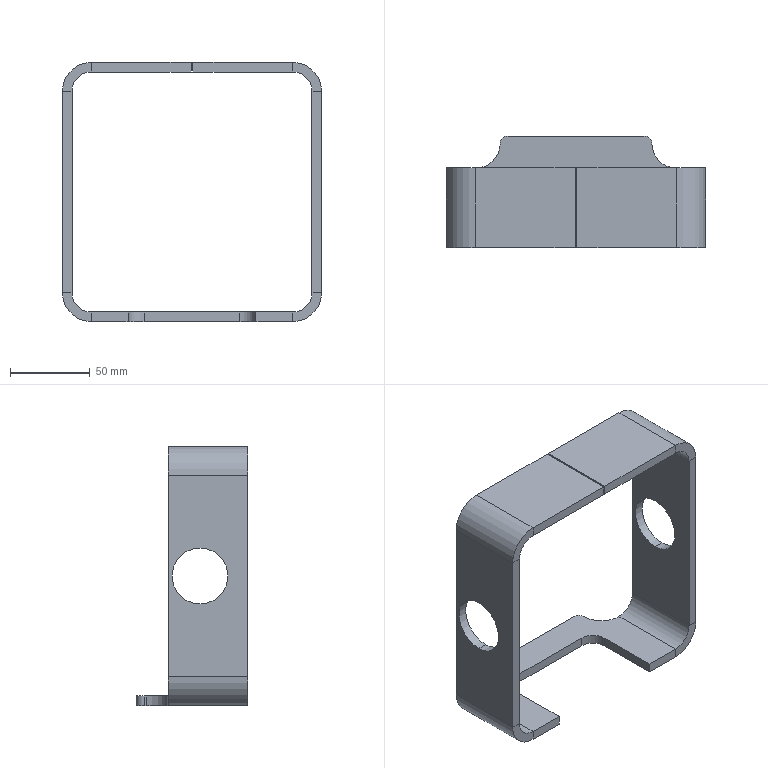Part | SolidWorks | features ICE 2, Fillet 1, FlatPattern 1, SMBaseFlange 1, SheetMetal 1 | 1 solid | 58 faces | box 162 x 70 x 162 mm | volume 155802 mm3 | plane 36 | cylinder 20 | spline 2 | commonest cylinder face diameters 24 x4 30 x4 35 x4 36 x4 10 x2 20 x2